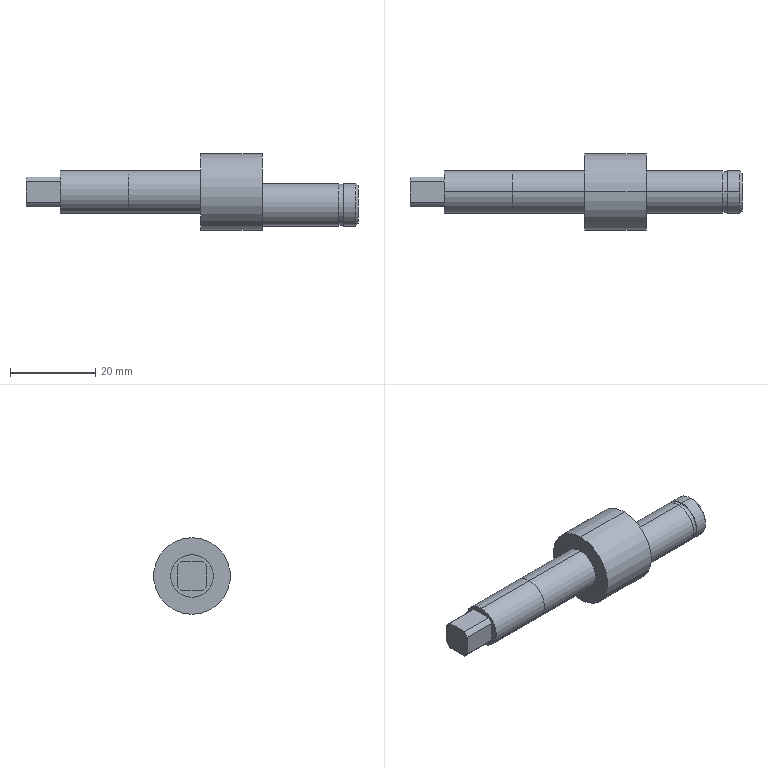Part | SolidWorks | features ICE 6, Chamfer 1, Extrusion 1 | 2 solids | 31 faces | box 78 x 18 x 18 mm | volume 8414 mm3 | cylinder 16 | plane 13 | cone 2 | commonest cylinder face diameters 10 x8 8.5 x4 9.6 x2 18 x2
STEP:
#1=CARTESIAN_POINT('',(-17.,0.,5.));
#2=VERTEX_POINT('',#1);
#3=CARTESIAN_POINT('',(-17.,0.,-5.));
#4=VERTEX_POINT('',#3);
#5=CARTESIAN_POINT('',(-17.,0.,0.));
#6=DIRECTION('',(-1.,0.,0.));
#7=DIRECTION('',(0.,0.,1.));
#8=AXIS2_PLACEMENT_3D('',#5,#6,#7);
#9=CIRCLE('',#8,5.);
#10=EDGE_CURVE('',#2,#4,#9,.T.);
#11=ORIENTED_EDGE('',*,*,#10,.F.);
#12=CARTESIAN_POINT('',(0.,0.,5.));
#13=VERTEX_POINT('',#12);
#14=CARTESIAN_POINT('',(-17.,0.,5.));
#15=DIRECTION('',(1.,0.,0.));
#16=VECTOR('',#15,1000.);
#17=LINE('',#14,#16);
#18=EDGE_CURVE('',#2,#13,#17,.T.);
#19=ORIENTED_EDGE('',*,*,#18,.T.);
#20=CARTESIAN_POINT('',(0.,0.,-5.));
#21=VERTEX_POINT('',#20);
#22=CARTESIAN_POINT('',(0.,0.,0.));
#23=DIRECTION('',(-1.,0.,0.));
#24=DIRECTION('',(0.,0.,1.));
#25=AXIS2_PLACEMENT_3D('',#22,#23,#24);
#26=CIRCLE('',#25,5.);
#27=EDGE_CURVE('',#13,#21,#26,.T.);
#28=ORIENTED_EDGE('',*,*,#27,.T.);
#29=CARTESIAN_POINT('',(-17.,0.,-5.));
#30=DIRECTION('',(1.,0.,0.));
#31=VECTOR('',#30,1000.);
#32=LINE('',#29,#31);
#33=EDGE_CURVE('',#4,#21,#32,.T.);
#34=ORIENTED_EDGE('',*,*,#33,.F.);
#35=EDGE_LOOP('',(#11,#19,#28,#34));
#36=FACE_OUTER_BOUND('',#35,.T.);
#37=CARTESIAN_POINT('',(-17.,0.,0.));
#38=DIRECTION('',(1.,0.,0.));
#39=DIRECTION('',(0.,0.,-1.));
#40=AXIS2_PLACEMENT_3D('',#37,#38,#39);
#41=CYLINDRICAL_SURFACE('',#40,5.);
#42=ADVANCED_FACE('',(#36),#41,.T.);
#43=CARTESIAN_POINT('',(37.,0.,-7.5));
#44=VERTEX_POINT('',#43);
#45=CARTESIAN_POINT('',(37.,0.,1.5));
#46=VERTEX_POINT('',#45);
#47=CARTESIAN_POINT('',(37.,0.,-3.));
#48=DIRECTION('',(1.,0.,0.));
#49=DIRECTION('',(0.,0.,-1.));
#50=AXIS2_PLACEMENT_3D('',#47,#48,#49);
#51=CIRCLE('',#50,4.5);
#52=EDGE_CURVE('',#44,#46,#51,.T.);
#53=ORIENTED_EDGE('',*,*,#52,.F.);
#54=CARTESIAN_POINT('',(36.5,0.,-8.));
#55=VERTEX_POINT('',#54);
#56=CARTESIAN_POINT('',(37.,0.,-7.5));
#57=DIRECTION('',(-0.7071,0.,-0.7071));
#58=VECTOR('',#57,1000.);
#59=LINE('',#56,#58);
#60=EDGE_CURVE('',#44,#55,#59,.T.);
#61=ORIENTED_EDGE('',*,*,#60,.T.);
#62=CARTESIAN_POINT('',(36.5,0.,2.));
#63=VERTEX_POINT('',#62);
#64=CARTESIAN_POINT('',(36.5,0.,-3.));
#65=DIRECTION('',(-1.,0.,0.));
#66=DIRECTION('',(0.,0.,-1.));
#67=AXIS2_PLACEMENT_3D('',#64,#65,#66);
#68=CIRCLE('',#67,5.);
#69=EDGE_CURVE('',#63,#55,#68,.T.);
#70=ORIENTED_EDGE('',*,*,#69,.F.);
#71=CARTESIAN_POINT('',(37.,0.,1.5));
#72=DIRECTION('',(-0.7071,0.,0.7071));
#73=VECTOR('',#72,1000.);
#74=LINE('',#71,#73);
#75=EDGE_CURVE('',#46,#63,#74,.T.);
#76=ORIENTED_EDGE('',*,*,#75,.F.);
#77=EDGE_LOOP('',(#53,#61,#70,#76));
#78=FACE_OUTER_BOUND('',#77,.T.);
#79=CARTESIAN_POINT('',(37.,0.,-3.));
#80=DIRECTION('',(-1.,0.,0.));
#81=DIRECTION('',(0.,0.,1.));
#82=AXIS2_PLACEMENT_3D('',#79,#80,#81);
#83=CONICAL_SURFACE('',#82,4.5,0.7854);
#84=ADVANCED_FACE('',(#78),#83,.T.);
#85=ORIENTED_EDGE('',*,*,#69,.T.);
#86=CARTESIAN_POINT('',(33.6,0.,-8.));
#87=VERTEX_POINT('',#86);
#88=CARTESIAN_POINT('',(37.,0.,-8.));
#89=DIRECTION('',(-1.,0.,0.));
#90=VECTOR('',#89,1000.);
#91=LINE('',#88,#90);
#92=EDGE_CURVE('',#55,#87,#91,.T.);
#93=ORIENTED_EDGE('',*,*,#92,.T.);
#94=CARTESIAN_POINT('',(33.6,0.,2.));
#95=VERTEX_POINT('',#94);
#96=CARTESIAN_POINT('',(33.6,0.,-3.));
#97=DIRECTION('',(1.,0.,0.));
#98=DIRECTION('',(0.,0.,-1.));
#99=AXIS2_PLACEMENT_3D('',#96,#97,#98);
#100=CIRCLE('',#99,5.);
#101=EDGE_CURVE('',#87,#95,#100,.T.);
#102=ORIENTED_EDGE('',*,*,#101,.T.);
#103=CARTESIAN_POINT('',(37.,0.,2.));
#104=DIRECTION('',(-1.,0.,0.));
#105=VECTOR('',#104,1000.);
#106=LINE('',#103,#105);
#107=EDGE_CURVE('',#63,#95,#106,.T.);
#108=ORIENTED_EDGE('',*,*,#107,.F.);
#109=EDGE_LOOP('',(#85,#93,#102,#108));
#110=FACE_OUTER_BOUND('',#109,.T.);
#111=CARTESIAN_POINT('',(37.,0.,-3.));
#112=DIRECTION('',(-1.,0.,0.));
#113=DIRECTION('',(0.,0.,1.));
#114=AXIS2_PLACEMENT_3D('',#111,#112,#113);
#115=CYLINDRICAL_SURFACE('',#114,5.);
#116=ADVANCED_FACE('',(#110),#115,.T.);
#117=CARTESIAN_POINT('',(33.6,0.,-7.8));
#118=VERTEX_POINT('',#117);
#119=CARTESIAN_POINT('',(33.6,0.,1.8));
#120=VERTEX_POINT('',#119);
#121=CARTESIAN_POINT('',(33.6,0.,-3.));
#122=DIRECTION('',(1.,0.,0.));
#123=DIRECTION('',(0.,0.,-1.));
#124=AXIS2_PLACEMENT_3D('',#121,#122,#123);
#125=CIRCLE('',#124,4.8);
#126=EDGE_CURVE('',#118,#120,#125,.T.);
#127=ORIENTED_EDGE('',*,*,#126,.F.);
#128=CARTESIAN_POINT('',(32.5,0.,-7.8));
#129=VERTEX_POINT('',#128);
#130=CARTESIAN_POINT('',(33.6,0.,-7.8));
#131=DIRECTION('',(-1.,0.,0.));
#132=VECTOR('',#131,1000.);
#133=LINE('',#130,#132);
#134=EDGE_CURVE('',#118,#129,#133,.T.);
#135=ORIENTED_EDGE('',*,*,#134,.T.);
#136=CARTESIAN_POINT('',(32.5,0.,1.8));
#137=VERTEX_POINT('',#136);
#138=CARTESIAN_POINT('',(32.5,0.,-3.));
#139=DIRECTION('',(1.,0.,0.));
#140=DIRECTION('',(0.,0.,-1.));
#141=AXIS2_PLACEMENT_3D('',#138,#139,#140);
#142=CIRCLE('',#141,4.8);
#143=EDGE_CURVE('',#129,#137,#142,.T.);
#144=ORIENTED_EDGE('',*,*,#143,.T.);
#145=CARTESIAN_POINT('',(33.6,0.,1.8));
#146=DIRECTION('',(-1.,0.,0.));
#147=VECTOR('',#146,1000.);
#148=LINE('',#145,#147);
#149=EDGE_CURVE('',#120,#137,#148,.T.);
#150=ORIENTED_EDGE('',*,*,#149,.F.);
#151=EDGE_LOOP('',(#127,#135,#144,#150));
#152=FACE_OUTER_BOUND('',#151,.T.);
#153=CARTESIAN_POINT('',(33.6,0.,-3.));
#154=DIRECTION('',(-1.,0.,0.));
#155=DIRECTION('',(0.,0.,1.));
#156=AXIS2_PLACEMENT_3D('',#153,#154,#155);
#157=CYLINDRICAL_SURFACE('',#156,4.8);
#158=ADVANCED_FACE('',(#152),#157,.T.);
#159=CARTESIAN_POINT('',(32.5,0.,-8.));
#160=VERTEX_POINT('',#159);
#161=CARTESIAN_POINT('',(32.5,0.,2.));
#162=VERTEX_POINT('',#161);
#163=CARTESIAN_POINT('',(32.5,0.,-3.));
#164=DIRECTION('',(1.,0.,0.));
#165=DIRECTION('',(0.,0.,-1.));
#166=AXIS2_PLACEMENT_3D('',#163,#164,#165);
#167=CIRCLE('',#166,5.);
#168=EDGE_CURVE('',#160,#162,#167,.T.);
#169=ORIENTED_EDGE('',*,*,#168,.F.);
#170=CARTESIAN_POINT('',(14.5,0.,-8.));
#171=VERTEX_POINT('',#170);
#172=CARTESIAN_POINT('',(32.5,0.,-8.));
#173=DIRECTION('',(-1.,0.,0.));
#174=VECTOR('',#173,1000.);
#175=LINE('',#172,#174);
#176=EDGE_CURVE('',#160,#171,#175,.T.);
#177=ORIENTED_EDGE('',*,*,#176,.T.);
#178=CARTESIAN_POINT('',(14.5,0.,2.));
#179=VERTEX_POINT('',#178);
#180=CARTESIAN_POINT('',(14.5,0.,-3.));
#181=DIRECTION('',(1.,0.,0.));
#182=DIRECTION('',(0.,0.,-1.));
#183=AXIS2_PLACEMENT_3D('',#180,#181,#182);
#184=CIRCLE('',#183,5.);
#185=EDGE_CURVE('',#171,#179,#184,.T.);
#186=ORIENTED_EDGE('',*,*,#185,.T.);
#187=CARTESIAN_POINT('',(32.5,0.,2.));
#188=DIRECTION('',(-1.,0.,0.));
#189=VECTOR('',#188,1000.);
#190=LINE('',#187,#189);
#191=EDGE_CURVE('',#162,#179,#190,.T.);
#192=ORIENTED_EDGE('',*,*,#191,.F.);
#193=EDGE_LOOP('',(#169,#177,#186,#192));
#194=FACE_OUTER_BOUND('',#193,.T.);
#195=CARTESIAN_POINT('',(32.5,0.,-3.));
#196=DIRECTION('',(-1.,0.,0.));
#197=DIRECTION('',(0.,0.,1.));
#198=AXIS2_PLACEMENT_3D('',#195,#196,#197);
#199=CYLINDRICAL_SURFACE('',#198,5.);
#200=ADVANCED_FACE('',(#194),#199,.T.);
#201=CARTESIAN_POINT('',(14.5,0.,-9.));
#202=VERTEX_POINT('',#201);
#203=CARTESIAN_POINT('',(14.5,0.,9.));
#204=VERTEX_POINT('',#203);
#205=CARTESIAN_POINT('',(14.5,0.,0.));
#206=DIRECTION('',(1.,0.,0.));
#207=DIRECTION('',(0.,0.,-1.));
#208=AXIS2_PLACEMENT_3D('',#205,#206,#207);
#209=CIRCLE('',#208,9.);
#210=EDGE_CURVE('',#202,#204,#209,.T.);
#211=ORIENTED_EDGE('',*,*,#210,.F.);
#212=CARTESIAN_POINT('',(0.,0.,-9.));
#213=VERTEX_POINT('',#212);
#214=CARTESIAN_POINT('',(14.5,0.,-9.));
#215=DIRECTION('',(-1.,0.,0.));
#216=VECTOR('',#215,1000.);
#217=LINE('',#214,#216);
#218=EDGE_CURVE('',#202,#213,#217,.T.);
#219=ORIENTED_EDGE('',*,*,#218,.T.);
#220=CARTESIAN_POINT('',(0.,0.,9.));
#221=VERTEX_POINT('',#220);
#222=CARTESIAN_POINT('',(0.,0.,0.));
#223=DIRECTION('',(1.,0.,0.));
#224=DIRECTION('',(0.,0.,-1.));
#225=AXIS2_PLACEMENT_3D('',#222,#223,#224);
#226=CIRCLE('',#225,9.);
#227=EDGE_CURVE('',#213,#221,#226,.T.);
#228=ORIENTED_EDGE('',*,*,#227,.T.);
#229=CARTESIAN_POINT('',(14.5,0.,9.));
#230=DIRECTION('',(-1.,0.,0.));
#231=VECTOR('',#230,1000.);
#232=LINE('',#229,#231);
#233=EDGE_CURVE('',#204,#221,#232,.T.);
#234=ORIENTED_EDGE('',*,*,#233,.F.);
#235=EDGE_LOOP('',(#211,#219,#228,#234));
#236=FACE_OUTER_BOUND('',#235,.T.);
#237=CARTESIAN_POINT('',(14.5,0.,0.));
#238=DIRECTION('',(-1.,0.,0.));
#239=DIRECTION('',(0.,0.,1.));
#240=AXIS2_PLACEMENT_3D('',#237,#238,#239);
#241=CYLINDRICAL_SURFACE('',#240,9.);
#242=ADVANCED_FACE('',(#236),#241,.T.);
#243=ORIENTED_EDGE('',*,*,#218,.F.);
#244=CARTESIAN_POINT('',(14.5,0.,0.));
#245=DIRECTION('',(1.,0.,0.));
#246=DIRECTION('',(0.,0.,-1.));
#247=AXIS2_PLACEMENT_3D('',#244,#245,#246);
#248=CIRCLE('',#247,9.);
#249=EDGE_CURVE('',#204,#202,#248,.T.);
#250=ORIENTED_EDGE('',*,*,#249,.F.);
#251=ORIENTED_EDGE('',*,*,#233,.T.);
#252=CARTESIAN_POINT('',(0.,0.,0.));
#253=DIRECTION('',(1.,0.,0.));
#254=DIRECTION('',(0.,0.,-1.));
#255=AXIS2_PLACEMENT_3D('',#252,#253,#254);
#256=CIRCLE('',#255,9.);
#257=EDGE_CURVE('',#221,#213,#256,.T.);
#258=ORIENTED_EDGE('',*,*,#257,.T.);
#259=EDGE_LOOP('',(#243,#250,#251,#258));
#260=FACE_OUTER_BOUND('',#259,.T.);
#261=CARTESIAN_POINT('',(14.5,0.,0.));
#262=DIRECTION('',(-1.,0.,0.));
#263=DIRECTION('',(0.,0.,1.));
#264=AXIS2_PLACEMENT_3D('',#261,#262,#263);
#265=CYLINDRICAL_SURFACE('',#264,9.);
#266=ADVANCED_FACE('',(#260),#265,.T.);
#267=CARTESIAN_POINT('',(14.5,0.,-3.));
#268=DIRECTION('',(1.,0.,0.));
#269=DIRECTION('',(0.,0.,-1.));
#270=AXIS2_PLACEMENT_3D('',#267,#268,#269);
#271=CIRCLE('',#270,5.);
#272=EDGE_CURVE('',#179,#171,#271,.T.);
#273=ORIENTED_EDGE('',*,*,#272,.F.);
#274=ORIENTED_EDGE('',*,*,#185,.F.);
#275=EDGE_LOOP('',(#273,#274));
#276=FACE_BOUND('',#275,.T.);
#277=ORIENTED_EDGE('',*,*,#249,.T.);
#278=ORIENTED_EDGE('',*,*,#210,.T.);
#279=EDGE_LOOP('',(#277,#278));
#280=FACE_OUTER_BOUND('',#279,.T.);
#281=CARTESIAN_POINT('',(14.5,0.,0.));
#282=DIRECTION('',(1.,0.,0.));
#283=DIRECTION('',(0.,0.,-1.));
#284=AXIS2_PLACEMENT_3D('',#281,#282,#283);
#285=PLANE('',#284);
#286=ADVANCED_FACE('',(#276,#280),#285,.T.);
#287=CARTESIAN_POINT('',(0.,0.,0.));
#288=DIRECTION('',(-1.,0.,0.));
#289=DIRECTION('',(0.,0.,1.));
#290=AXIS2_PLACEMENT_3D('',#287,#288,#289);
#291=CIRCLE('',#290,5.);
#292=EDGE_CURVE('',#21,#13,#291,.T.);
#293=ORIENTED_EDGE('',*,*,#292,.F.);
#294=ORIENTED_EDGE('',*,*,#27,.F.);
#295=EDGE_LOOP('',(#293,#294));
#296=FACE_BOUND('',#295,.T.);
#297=ORIENTED_EDGE('',*,*,#257,.F.);
#298=ORIENTED_EDGE('',*,*,#227,.F.);
#299=EDGE_LOOP('',(#297,#298));
#300=FACE_OUTER_BOUND('',#299,.T.);
#301=CARTESIAN_POINT('',(0.,0.,0.));
#302=DIRECTION('',(1.,0.,0.));
#303=DIRECTION('',(0.,0.,-1.));
#304=AXIS2_PLACEMENT_3D('',#301,#302,#303);
#305=PLANE('',#304);
#306=ADVANCED_FACE('',(#296,#300),#305,.F.);
#307=ORIENTED_EDGE('',*,*,#176,.F.);
#308=CARTESIAN_POINT('',(32.5,0.,-3.));
#309=DIRECTION('',(1.,0.,0.));
#310=DIRECTION('',(0.,0.,-1.));
#311=AXIS2_PLACEMENT_3D('',#308,#309,#310);
#312=CIRCLE('',#311,5.);
#313=EDGE_CURVE('',#162,#160,#312,.T.);
#314=ORIENTED_EDGE('',*,*,#313,.F.);
#315=ORIENTED_EDGE('',*,*,#191,.T.);
#316=ORIENTED_EDGE('',*,*,#272,.T.);
#317=EDGE_LOOP('',(#307,#314,#315,#316));
#318=FACE_OUTER_BOUND('',#317,.T.);
#319=CARTESIAN_POINT('',(32.5,0.,-3.));
#320=DIRECTION('',(-1.,0.,0.));
#321=DIRECTION('',(0.,0.,1.));
#322=AXIS2_PLACEMENT_3D('',#319,#320,#321);
#323=CYLINDRICAL_SURFACE('',#322,5.);
#324=ADVANCED_FACE('',(#318),#323,.T.);
#325=CARTESIAN_POINT('',(32.5,0.,-3.));
#326=DIRECTION('',(1.,0.,0.));
#327=DIRECTION('',(0.,0.,-1.));
#328=AXIS2_PLACEMENT_3D('',#325,#326,#327);
#329=CIRCLE('',#328,4.8);
#330=EDGE_CURVE('',#137,#129,#329,.T.);
#331=ORIENTED_EDGE('',*,*,#330,.F.);
#332=ORIENTED_EDGE('',*,*,#143,.F.);
#333=EDGE_LOOP('',(#331,#332));
#334=FACE_BOUND('',#333,.T.);
#335=ORIENTED_EDGE('',*,*,#313,.T.);
#336=ORIENTED_EDGE('',*,*,#168,.T.);
#337=EDGE_LOOP('',(#335,#336));
#338=FACE_OUTER_BOUND('',#337,.T.);
#339=CARTESIAN_POINT('',(32.5,0.,-3.));
#340=DIRECTION('',(1.,0.,0.));
#341=DIRECTION('',(0.,0.,-1.));
#342=AXIS2_PLACEMENT_3D('',#339,#340,#341);
#343=PLANE('',#342);
#344=ADVANCED_FACE('',(#334,#338),#343,.T.);
#345=ORIENTED_EDGE('',*,*,#134,.F.);
#346=CARTESIAN_POINT('',(33.6,0.,-3.));
#347=DIRECTION('',(1.,0.,0.));
#348=DIRECTION('',(0.,0.,-1.));
#349=AXIS2_PLACEMENT_3D('',#346,#347,#348);
#350=CIRCLE('',#349,4.8);
#351=EDGE_CURVE('',#120,#118,#350,.T.);
#352=ORIENTED_EDGE('',*,*,#351,.F.);
#353=ORIENTED_EDGE('',*,*,#149,.T.);
#354=ORIENTED_EDGE('',*,*,#330,.T.);
#355=EDGE_LOOP('',(#345,#352,#353,#354));
#356=FACE_OUTER_BOUND('',#355,.T.);
#357=CARTESIAN_POINT('',(33.6,0.,-3.));
#358=DIRECTION('',(-1.,0.,0.));
#359=DIRECTION('',(0.,0.,1.));
#360=AXIS2_PLACEMENT_3D('',#357,#358,#359);
#361=CYLINDRICAL_SURFACE('',#360,4.8);
#362=ADVANCED_FACE('',(#356),#361,.T.);
#363=ORIENTED_EDGE('',*,*,#92,.F.);
#364=CARTESIAN_POINT('',(36.5,0.,-3.));
#365=DIRECTION('',(-1.,0.,0.));
#366=DIRECTION('',(0.,0.,-1.));
#367=AXIS2_PLACEMENT_3D('',#364,#365,#366);
#368=CIRCLE('',#367,5.);
#369=EDGE_CURVE('',#55,#63,#368,.T.);
#370=ORIENTED_EDGE('',*,*,#369,.T.);
#371=ORIENTED_EDGE('',*,*,#107,.T.);
#372=CARTESIAN_POINT('',(33.6,0.,-3.));
#373=DIRECTION('',(1.,0.,0.));
#374=DIRECTION('',(0.,0.,-1.));
#375=AXIS2_PLACEMENT_3D('',#372,#373,#374);
#376=CIRCLE('',#375,5.);
#377=EDGE_CURVE('',#95,#87,#376,.T.);
#378=ORIENTED_EDGE('',*,*,#377,.T.);
#379=EDGE_LOOP('',(#363,#370,#371,#378));
#380=FACE_OUTER_BOUND('',#379,.T.);
#381=CARTESIAN_POINT('',(37.,0.,-3.));
#382=DIRECTION('',(-1.,0.,0.));
#383=DIRECTION('',(0.,0.,1.));
#384=AXIS2_PLACEMENT_3D('',#381,#382,#383);
#385=CYLINDRICAL_SURFACE('',#384,5.);
#386=ADVANCED_FACE('',(#380),#385,.T.);
#387=CARTESIAN_POINT('',(37.,0.,-3.));
#388=DIRECTION('',(1.,0.,0.));
#389=DIRECTION('',(0.,0.,-1.));
#390=AXIS2_PLACEMENT_3D('',#387,#388,#389);
#391=CIRCLE('',#390,4.5);
#392=EDGE_CURVE('',#46,#44,#391,.T.);
#393=ORIENTED_EDGE('',*,*,#392,.T.);
#394=ORIENTED_EDGE('',*,*,#52,.T.);
#395=EDGE_LOOP('',(#393,#394));
#396=FACE_OUTER_BOUND('',#395,.T.);
#397=CARTESIAN_POINT('',(37.,0.,-3.));
#398=DIRECTION('',(1.,0.,0.));
#399=DIRECTION('',(0.,0.,-1.));
#400=AXIS2_PLACEMENT_3D('',#397,#398,#399);
#401=PLANE('',#400);
#402=ADVANCED_FACE('',(#396),#401,.T.);
#403=ORIENTED_EDGE('',*,*,#351,.T.);
#404=ORIENTED_EDGE('',*,*,#126,.T.);
#405=EDGE_LOOP('',(#403,#404));
#406=FACE_BOUND('',#405,.T.);
#407=ORIENTED_EDGE('',*,*,#377,.F.);
#408=ORIENTED_EDGE('',*,*,#101,.F.);
#409=EDGE_LOOP('',(#407,#408));
#410=FACE_OUTER_BOUND('',#409,.T.);
#411=CARTESIAN_POINT('',(33.6,0.,-3.));
#412=DIRECTION('',(1.,0.,0.));
#413=DIRECTION('',(0.,0.,-1.));
#414=AXIS2_PLACEMENT_3D('',#411,#412,#413);
#415=PLANE('',#414);
#416=ADVANCED_FACE('',(#406,#410),#415,.F.);
#417=ORIENTED_EDGE('',*,*,#60,.F.);
#418=ORIENTED_EDGE('',*,*,#392,.F.);
#419=ORIENTED_EDGE('',*,*,#75,.T.);
#420=ORIENTED_EDGE('',*,*,#369,.F.);
#421=EDGE_LOOP('',(#417,#418,#419,#420));
#422=FACE_OUTER_BOUND('',#421,.T.);
#423=CARTESIAN_POINT('',(37.,0.,-3.));
#424=DIRECTION('',(-1.,0.,0.));
#425=DIRECTION('',(0.,0.,1.));
#426=AXIS2_PLACEMENT_3D('',#423,#424,#425);
#427=CONICAL_SURFACE('',#426,4.5,0.7854);
#428=ADVANCED_FACE('',(#422),#427,.T.);
#429=ORIENTED_EDGE('',*,*,#18,.F.);
#430=CARTESIAN_POINT('',(-17.,0.,0.));
#431=DIRECTION('',(-1.,0.,0.));
#432=DIRECTION('',(0.,0.,1.));
#433=AXIS2_PLACEMENT_3D('',#430,#431,#432);
#434=CIRCLE('',#433,5.);
#435=EDGE_CURVE('',#4,#2,#434,.T.);
#436=ORIENTED_EDGE('',*,*,#435,.F.);
#437=ORIENTED_EDGE('',*,*,#33,.T.);
#438=ORIENTED_EDGE('',*,*,#292,.T.);
#439=EDGE_LOOP('',(#429,#436,#437,#438));
#440=FACE_OUTER_BOUND('',#439,.T.);
#441=CARTESIAN_POINT('',(-17.,0.,0.));
#442=DIRECTION('',(1.,0.,0.));
#443=DIRECTION('',(0.,0.,-1.));
#444=AXIS2_PLACEMENT_3D('',#441,#442,#443);
#445=CYLINDRICAL_SURFACE('',#444,5.);
#446=ADVANCED_FACE('',(#440),#445,.T.);
#447=ORIENTED_EDGE('',*,*,#435,.T.);
#448=ORIENTED_EDGE('',*,*,#10,.T.);
#449=EDGE_LOOP('',(#447,#448));
#450=FACE_OUTER_BOUND('',#449,.T.);
#451=CARTESIAN_POINT('',(-17.,0.,0.));
#452=DIRECTION('',(-1.,0.,0.));
#453=DIRECTION('',(0.,0.,1.));
#454=AXIS2_PLACEMENT_3D('',#451,#452,#453);
#455=PLANE('',#454);
#456=ADVANCED_FACE('',(#450),#455,.T.);
#457=CLOSED_SHELL('',(#42,#84,#116,#158,#200,#242,#266,#286,#306,#324,#344,#362,#386,#402,#416,#428,#446,#456));
#458=MANIFOLD_SOLID_BREP('',#457);
#459=CARTESIAN_POINT('',(-33.,0.,5.));
#460=VERTEX_POINT('',#459);
#461=CARTESIAN_POINT('',(-33.,0.,-5.));
#462=VERTEX_POINT('',#461);
#463=CARTESIAN_POINT('',(-33.,0.,0.));
#464=DIRECTION('',(-1.,0.,0.));
#465=DIRECTION('',(0.,0.,1.));
#466=AXIS2_PLACEMENT_3D('',#463,#464,#465);
#467=CIRCLE('',#466,5.);
#468=EDGE_CURVE('',#460,#462,#467,.T.);
#469=ORIENTED_EDGE('',*,*,#468,.F.);
#470=CARTESIAN_POINT('',(-17.,0.,5.));
#471=VERTEX_POINT('',#470);
#472=CARTESIAN_POINT('',(-33.,0.,5.));
#473=DIRECTION('',(1.,0.,0.));
#474=VECTOR('',#473,1000.);
#475=LINE('',#472,#474);
#476=EDGE_CURVE('',#460,#471,#475,.T.);
#477=ORIENTED_EDGE('',*,*,#476,.T.);
#478=CARTESIAN_POINT('',(-17.,0.,-5.));
#479=VERTEX_POINT('',#478);
#480=CARTESIAN_POINT('',(-17.,0.,0.));
#481=DIRECTION('',(-1.,0.,0.));
#482=DIRECTION('',(0.,0.,1.));
#483=AXIS2_PLACEMENT_3D('',#480,#481,#482);
#484=CIRCLE('',#483,5.);
#485=EDGE_CURVE('',#471,#479,#484,.T.);
#486=ORIENTED_EDGE('',*,*,#485,.T.);
#487=CARTESIAN_POINT('',(-33.,0.,-5.));
#488=DIRECTION('',(1.,0.,0.));
#489=VECTOR('',#488,1000.);
#490=LINE('',#487,#489);
#491=EDGE_CURVE('',#462,#479,#490,.T.);
#492=ORIENTED_EDGE('',*,*,#491,.F.);
#493=EDGE_LOOP('',(#469,#477,#486,#492));
#494=FACE_OUTER_BOUND('',#493,.T.);
#495=CARTESIAN_POINT('',(-33.,0.,0.));
#496=DIRECTION('',(1.,0.,0.));
#497=DIRECTION('',(0.,0.,-1.));
#498=AXIS2_PLACEMENT_3D('',#495,#496,#497);
#499=CYLINDRICAL_SURFACE('',#498,5.);
#500=ADVANCED_FACE('',(#494),#499,.T.);
#501=ORIENTED_EDGE('',*,*,#476,.F.);
#502=CARTESIAN_POINT('',(-33.,0.,0.));
#503=DIRECTION('',(-1.,0.,0.));
#504=DIRECTION('',(0.,0.,1.));
#505=AXIS2_PLACEMENT_3D('',#502,#503,#504);
#506=CIRCLE('',#505,5.);
#507=EDGE_CURVE('',#462,#460,#506,.T.);
#508=ORIENTED_EDGE('',*,*,#507,.F.);
#509=ORIENTED_EDGE('',*,*,#491,.T.);
#510=CARTESIAN_POINT('',(-17.,0.,0.));
#511=DIRECTION('',(-1.,0.,0.));
#512=DIRECTION('',(0.,0.,1.));
#513=AXIS2_PLACEMENT_3D('',#510,#511,#512);
#514=CIRCLE('',#513,5.);
#515=EDGE_CURVE('',#479,#471,#514,.T.);
#516=ORIENTED_EDGE('',*,*,#515,.T.);
#517=EDGE_LOOP('',(#501,#508,#509,#516));
#518=FACE_OUTER_BOUND('',#517,.T.);
#519=CARTESIAN_POINT('',(-33.,0.,0.));
#520=DIRECTION('',(1.,0.,0.));
#521=DIRECTION('',(0.,0.,-1.));
#522=AXIS2_PLACEMENT_3D('',#519,#520,#521);
#523=CYLINDRICAL_SURFACE('',#522,5.);
#524=ADVANCED_FACE('',(#518),#523,.T.);
#525=CARTESIAN_POINT('',(-33.,3.5,-2.411));
#526=VERTEX_POINT('',#525);
#527=CARTESIAN_POINT('',(-33.,2.411,-3.5));
#528=VERTEX_POINT('',#527);
#529=CARTESIAN_POINT('',(-33.,0.,0.));
#530=DIRECTION('',(-1.,0.,0.));
#531=DIRECTION('',(0.,0.,1.));
#532=AXIS2_PLACEMENT_3D('',#529,#530,#531);
#533=CIRCLE('',#532,4.25);
#534=EDGE_CURVE('',#526,#528,#533,.T.);
#535=ORIENTED_EDGE('',*,*,#534,.F.);
#536=CARTESIAN_POINT('',(-33.,3.5,2.411));
#537=VERTEX_POINT('',#536);
#538=CARTESIAN_POINT('',(-33.,3.5,-2.411));
#539=DIRECTION('',(0.,0.,-1.));
#540=VECTOR('',#539,1000.);
#541=LINE('',#538,#540);
#542=EDGE_CURVE('',#537,#526,#541,.T.);
#543=ORIENTED_EDGE('',*,*,#542,.F.);
#544=CARTESIAN_POINT('',(-33.,2.411,3.5));
#545=VERTEX_POINT('',#544);
#546=CARTESIAN_POINT('',(-33.,0.,0.));
#547=DIRECTION('',(-1.,0.,0.));
#548=DIRECTION('',(0.,0.,1.));
#549=AXIS2_PLACEMENT_3D('',#546,#547,#548);
#550=CIRCLE('',#549,4.25);
#551=EDGE_CURVE('',#545,#537,#550,.T.);
#552=ORIENTED_EDGE('',*,*,#551,.F.);
#553=CARTESIAN_POINT('',(-33.,-2.411,3.5));
#554=VERTEX_POINT('',#553);
#555=CARTESIAN_POINT('',(-33.,-2.411,3.5));
#556=DIRECTION('',(0.,1.,0.));
#557=VECTOR('',#556,1000.);
#558=LINE('',#555,#557);
#559=EDGE_CURVE('',#554,#545,#558,.T.);
#560=ORIENTED_EDGE('',*,*,#559,.F.);
#561=CARTESIAN_POINT('',(-33.,-3.5,2.411));
#562=VERTEX_POINT('',#561);
#563=CARTESIAN_POINT('',(-33.,0.,0.));
#564=DIRECTION('',(-1.,0.,0.));
#565=DIRECTION('',(0.,0.,1.));
#566=AXIS2_PLACEMENT_3D('',#563,#564,#565);
#567=CIRCLE('',#566,4.25);
#568=EDGE_CURVE('',#562,#554,#567,.T.);
#569=ORIENTED_EDGE('',*,*,#568,.F.);
#570=CARTESIAN_POINT('',(-33.,-3.5,-2.411));
#571=VERTEX_POINT('',#570);
#572=CARTESIAN_POINT('',(-33.,-3.5,-2.411));
#573=DIRECTION('',(0.,0.,1.));
#574=VECTOR('',#573,1000.);
#575=LINE('',#572,#574);
#576=EDGE_CURVE('',#571,#562,#575,.T.);
#577=ORIENTED_EDGE('',*,*,#576,.F.);
#578=CARTESIAN_POINT('',(-33.,-2.411,-3.5));
#579=VERTEX_POINT('',#578);
#580=CARTESIAN_POINT('',(-33.,0.,0.));
#581=DIRECTION('',(-1.,0.,0.));
#582=DIRECTION('',(0.,0.,1.));
#583=AXIS2_PLACEMENT_3D('',#580,#581,#582);
#584=CIRCLE('',#583,4.25);
#585=EDGE_CURVE('',#579,#571,#584,.T.);
#586=ORIENTED_EDGE('',*,*,#585,.F.);
#587=CARTESIAN_POINT('',(-33.,-2.411,-3.5));
#588=DIRECTION('',(0.,-1.,0.));
#589=VECTOR('',#588,1000.);
#590=LINE('',#587,#589);
#591=EDGE_CURVE('',#528,#579,#590,.T.);
#592=ORIENTED_EDGE('',*,*,#591,.F.);
#593=EDGE_LOOP('',(#535,#543,#552,#560,#569,#577,#586,#592));
#594=FACE_BOUND('',#593,.T.);
#595=ORIENTED_EDGE('',*,*,#507,.T.);
#596=ORIENTED_EDGE('',*,*,#468,.T.);
#597=EDGE_LOOP('',(#595,#596));
#598=FACE_OUTER_BOUND('',#597,.T.);
#599=CARTESIAN_POINT('',(-33.,0.,0.));
#600=DIRECTION('',(-1.,0.,0.));
#601=DIRECTION('',(0.,0.,1.));
#602=AXIS2_PLACEMENT_3D('',#599,#600,#601);
#603=PLANE('',#602);
#604=ADVANCED_FACE('',(#594,#598),#603,.T.);
#605=ORIENTED_EDGE('',*,*,#515,.F.);
#606=ORIENTED_EDGE('',*,*,#485,.F.);
#607=EDGE_LOOP('',(#605,#606));
#608=FACE_OUTER_BOUND('',#607,.T.);
#609=CARTESIAN_POINT('',(-17.,0.,0.));
#610=DIRECTION('',(-1.,0.,0.));
#611=DIRECTION('',(0.,0.,1.));
#612=AXIS2_PLACEMENT_3D('',#609,#610,#611);
#613=PLANE('',#612);
#614=ADVANCED_FACE('',(#608),#613,.F.);
#615=ORIENTED_EDGE('',*,*,#534,.T.);
#616=CARTESIAN_POINT('',(-41.,2.411,-3.5));
#617=VERTEX_POINT('',#616);
#618=CARTESIAN_POINT('',(-41.,2.411,-3.5));
#619=DIRECTION('',(1.,0.,0.));
#620=VECTOR('',#619,1000.);
#621=LINE('',#618,#620);
#622=EDGE_CURVE('',#617,#528,#621,.T.);
#623=ORIENTED_EDGE('',*,*,#622,.F.);
#624=CARTESIAN_POINT('',(-41.,3.5,-2.411));
#625=VERTEX_POINT('',#624);
#626=CARTESIAN_POINT('',(-41.,0.,0.));
#627=DIRECTION('',(-1.,0.,0.));
#628=DIRECTION('',(0.,0.,1.));
#629=AXIS2_PLACEMENT_3D('',#626,#627,#628);
#630=CIRCLE('',#629,4.25);
#631=EDGE_CURVE('',#625,#617,#630,.T.);
#632=ORIENTED_EDGE('',*,*,#631,.F.);
#633=CARTESIAN_POINT('',(-41.,3.5,-2.411));
#634=DIRECTION('',(1.,0.,0.));
#635=VECTOR('',#634,1000.);
#636=LINE('',#633,#635);
#637=EDGE_CURVE('',#625,#526,#636,.T.);
#638=ORIENTED_EDGE('',*,*,#637,.T.);
#639=EDGE_LOOP('',(#615,#623,#632,#638));
#640=FACE_OUTER_BOUND('',#639,.T.);
#641=CARTESIAN_POINT('',(-41.,0.,0.));
#642=DIRECTION('',(1.,0.,0.));
#643=DIRECTION('',(0.,0.,-1.));
#644=AXIS2_PLACEMENT_3D('',#641,#642,#643);
#645=CYLINDRICAL_SURFACE('',#644,4.25);
#646=ADVANCED_FACE('',(#640),#645,.T.);
#647=ORIENTED_EDGE('',*,*,#591,.T.);
#648=CARTESIAN_POINT('',(-41.,-2.411,-3.5));
#649=VERTEX_POINT('',#648);
#650=CARTESIAN_POINT('',(-41.,-2.411,-3.5));
#651=DIRECTION('',(1.,0.,0.));
#652=VECTOR('',#651,1000.);
#653=LINE('',#650,#652);
#654=EDGE_CURVE('',#649,#579,#653,.T.);
#655=ORIENTED_EDGE('',*,*,#654,.F.);
#656=CARTESIAN_POINT('',(-41.,-2.411,-3.5));
#657=DIRECTION('',(0.,-1.,0.));
#658=VECTOR('',#657,1000.);
#659=LINE('',#656,#658);
#660=EDGE_CURVE('',#617,#649,#659,.T.);
#661=ORIENTED_EDGE('',*,*,#660,.F.);
#662=ORIENTED_EDGE('',*,*,#622,.T.);
#663=EDGE_LOOP('',(#647,#655,#661,#662));
#664=FACE_OUTER_BOUND('',#663,.T.);
#665=CARTESIAN_POINT('',(-41.,-2.411,-3.5));
#666=DIRECTION('',(0.,0.,1.));
#667=DIRECTION('',(1.,0.,0.));
#668=AXIS2_PLACEMENT_3D('',#665,#666,#667);
#669=PLANE('',#668);
#670=ADVANCED_FACE('',(#664),#669,.F.);
#671=ORIENTED_EDGE('',*,*,#585,.T.);
#672=CARTESIAN_POINT('',(-41.,-3.5,-2.411));
#673=VERTEX_POINT('',#672);
#674=CARTESIAN_POINT('',(-41.,-3.5,-2.411));
#675=DIRECTION('',(1.,0.,0.));
#676=VECTOR('',#675,1000.);
#677=LINE('',#674,#676);
#678=EDGE_CURVE('',#673,#571,#677,.T.);
#679=ORIENTED_EDGE('',*,*,#678,.F.);
#680=CARTESIAN_POINT('',(-41.,0.,0.));
#681=DIRECTION('',(-1.,0.,0.));
#682=DIRECTION('',(0.,0.,1.));
#683=AXIS2_PLACEMENT_3D('',#680,#681,#682);
#684=CIRCLE('',#683,4.25);
#685=EDGE_CURVE('',#649,#673,#684,.T.);
#686=ORIENTED_EDGE('',*,*,#685,.F.);
#687=ORIENTED_EDGE('',*,*,#654,.T.);
#688=EDGE_LOOP('',(#671,#679,#686,#687));
#689=FACE_OUTER_BOUND('',#688,.T.);
#690=CARTESIAN_POINT('',(-41.,0.,0.));
#691=DIRECTION('',(1.,0.,0.));
#692=DIRECTION('',(0.,0.,-1.));
#693=AXIS2_PLACEMENT_3D('',#690,#691,#692);
#694=CYLINDRICAL_SURFACE('',#693,4.25);
#695=ADVANCED_FACE('',(#689),#694,.T.);
#696=ORIENTED_EDGE('',*,*,#576,.T.);
#697=CARTESIAN_POINT('',(-41.,-3.5,2.411));
#698=VERTEX_POINT('',#697);
#699=CARTESIAN_POINT('',(-41.,-3.5,2.411));
#700=DIRECTION('',(1.,0.,0.));
#701=VECTOR('',#700,1000.);
#702=LINE('',#699,#701);
#703=EDGE_CURVE('',#698,#562,#702,.T.);
#704=ORIENTED_EDGE('',*,*,#703,.F.);
#705=CARTESIAN_POINT('',(-41.,-3.5,-2.411));
#706=DIRECTION('',(0.,0.,1.));
#707=VECTOR('',#706,1000.);
#708=LINE('',#705,#707);
#709=EDGE_CURVE('',#673,#698,#708,.T.);
#710=ORIENTED_EDGE('',*,*,#709,.F.);
#711=ORIENTED_EDGE('',*,*,#678,.T.);
#712=EDGE_LOOP('',(#696,#704,#710,#711));
#713=FACE_OUTER_BOUND('',#712,.T.);
#714=CARTESIAN_POINT('',(-41.,-3.5,-2.411));
#715=DIRECTION('',(0.,1.,0.));
#716=DIRECTION('',(0.,0.,1.));
#717=AXIS2_PLACEMENT_3D('',#714,#715,#716);
#718=PLANE('',#717);
#719=ADVANCED_FACE('',(#713),#718,.F.);
#720=ORIENTED_EDGE('',*,*,#568,.T.);
#721=CARTESIAN_POINT('',(-41.,-2.411,3.5));
#722=VERTEX_POINT('',#721);
#723=CARTESIAN_POINT('',(-41.,-2.411,3.5));
#724=DIRECTION('',(1.,0.,0.));
#725=VECTOR('',#724,1000.);
#726=LINE('',#723,#725);
#727=EDGE_CURVE('',#722,#554,#726,.T.);
#728=ORIENTED_EDGE('',*,*,#727,.F.);
#729=CARTESIAN_POINT('',(-41.,0.,0.));
#730=DIRECTION('',(-1.,0.,0.));
#731=DIRECTION('',(0.,0.,1.));
#732=AXIS2_PLACEMENT_3D('',#729,#730,#731);
#733=CIRCLE('',#732,4.25);
#734=EDGE_CURVE('',#698,#722,#733,.T.);
#735=ORIENTED_EDGE('',*,*,#734,.F.);
#736=ORIENTED_EDGE('',*,*,#703,.T.);
#737=EDGE_LOOP('',(#720,#728,#735,#736));
#738=FACE_OUTER_BOUND('',#737,.T.);
#739=CARTESIAN_POINT('',(-41.,0.,0.));
#740=DIRECTION('',(1.,0.,0.));
#741=DIRECTION('',(0.,0.,-1.));
#742=AXIS2_PLACEMENT_3D('',#739,#740,#741);
#743=CYLINDRICAL_SURFACE('',#742,4.25);
#744=ADVANCED_FACE('',(#738),#743,.T.);
#745=ORIENTED_EDGE('',*,*,#559,.T.);
#746=CARTESIAN_POINT('',(-41.,2.411,3.5));
#747=VERTEX_POINT('',#746);
#748=CARTESIAN_POINT('',(-41.,2.411,3.5));
#749=DIRECTION('',(1.,0.,0.));
#750=VECTOR('',#749,1000.);
#751=LINE('',#748,#750);
#752=EDGE_CURVE('',#747,#545,#751,.T.);
#753=ORIENTED_EDGE('',*,*,#752,.F.);
#754=CARTESIAN_POINT('',(-41.,-2.411,3.5));
#755=DIRECTION('',(0.,1.,0.));
#756=VECTOR('',#755,1000.);
#757=LINE('',#754,#756);
#758=EDGE_CURVE('',#722,#747,#757,.T.);
#759=ORIENTED_EDGE('',*,*,#758,.F.);
#760=ORIENTED_EDGE('',*,*,#727,.T.);
#761=EDGE_LOOP('',(#745,#753,#759,#760));
#762=FACE_OUTER_BOUND('',#761,.T.);
#763=CARTESIAN_POINT('',(-41.,-2.411,3.5));
#764=DIRECTION('',(0.,0.,-1.));
#765=DIRECTION('',(-1.,0.,0.));
#766=AXIS2_PLACEMENT_3D('',#763,#764,#765);
#767=PLANE('',#766);
#768=ADVANCED_FACE('',(#762),#767,.F.);
#769=ORIENTED_EDGE('',*,*,#551,.T.);
#770=CARTESIAN_POINT('',(-41.,3.5,2.411));
#771=VERTEX_POINT('',#770);
#772=CARTESIAN_POINT('',(-41.,3.5,2.411));
#773=DIRECTION('',(1.,0.,0.));
#774=VECTOR('',#773,1000.);
#775=LINE('',#772,#774);
#776=EDGE_CURVE('',#771,#537,#775,.T.);
#777=ORIENTED_EDGE('',*,*,#776,.F.);
#778=CARTESIAN_POINT('',(-41.,0.,0.));
#779=DIRECTION('',(-1.,0.,0.));
#780=DIRECTION('',(0.,0.,1.));
#781=AXIS2_PLACEMENT_3D('',#778,#779,#780);
#782=CIRCLE('',#781,4.25);
#783=EDGE_CURVE('',#747,#771,#782,.T.);
#784=ORIENTED_EDGE('',*,*,#783,.F.);
#785=ORIENTED_EDGE('',*,*,#752,.T.);
#786=EDGE_LOOP('',(#769,#777,#784,#785));
#787=FACE_OUTER_BOUND('',#786,.T.);
#788=CARTESIAN_POINT('',(-41.,0.,0.));
#789=DIRECTION('',(1.,0.,0.));
#790=DIRECTION('',(0.,0.,-1.));
#791=AXIS2_PLACEMENT_3D('',#788,#789,#790);
#792=CYLINDRICAL_SURFACE('',#791,4.25);
#793=ADVANCED_FACE('',(#787),#792,.T.);
#794=ORIENTED_EDGE('',*,*,#542,.T.);
#795=ORIENTED_EDGE('',*,*,#637,.F.);
#796=CARTESIAN_POINT('',(-41.,3.5,-2.411));
#797=DIRECTION('',(0.,0.,-1.));
#798=VECTOR('',#797,1000.);
#799=LINE('',#796,#798);
#800=EDGE_CURVE('',#771,#625,#799,.T.);
#801=ORIENTED_EDGE('',*,*,#800,.F.);
#802=ORIENTED_EDGE('',*,*,#776,.T.);
#803=EDGE_LOOP('',(#794,#795,#801,#802));
#804=FACE_OUTER_BOUND('',#803,.T.);
#805=CARTESIAN_POINT('',(-41.,3.5,-2.411));
#806=DIRECTION('',(0.,-1.,0.));
#807=DIRECTION('',(0.,0.,-1.));
#808=AXIS2_PLACEMENT_3D('',#805,#806,#807);
#809=PLANE('',#808);
#810=ADVANCED_FACE('',(#804),#809,.F.);
#811=ORIENTED_EDGE('',*,*,#631,.T.);
#812=ORIENTED_EDGE('',*,*,#660,.T.);
#813=ORIENTED_EDGE('',*,*,#685,.T.);
#814=ORIENTED_EDGE('',*,*,#709,.T.);
#815=ORIENTED_EDGE('',*,*,#734,.T.);
#816=ORIENTED_EDGE('',*,*,#758,.T.);
#817=ORIENTED_EDGE('',*,*,#783,.T.);
#818=ORIENTED_EDGE('',*,*,#800,.T.);
#819=EDGE_LOOP('',(#811,#812,#813,#814,#815,#816,#817,#818));
#820=FACE_OUTER_BOUND('',#819,.T.);
#821=CARTESIAN_POINT('',(-41.,0.,0.));
#822=DIRECTION('',(-1.,0.,0.));
#823=DIRECTION('',(0.,0.,1.));
#824=AXIS2_PLACEMENT_3D('',#821,#822,#823);
#825=PLANE('',#824);
#826=ADVANCED_FACE('',(#820),#825,.T.);
#827=CLOSED_SHELL('',(#500,#524,#604,#614,#646,#670,#695,#719,#744,#768,#793,#810,#826));
#828=MANIFOLD_SOLID_BREP('',#827);
#829=CARTESIAN_POINT('',(0.,0.,0.));
#830=DIRECTION('',(0.,0.,1.));
#831=DIRECTION('',(1.,0.,0.));
#832=AXIS2_PLACEMENT_3D('',#829,#830,#831);
#833=(LENGTH_UNIT()NAMED_UNIT(*)SI_UNIT(.MILLI.,.METRE.));
#834=UNCERTAINTY_MEASURE_WITH_UNIT(LENGTH_MEASURE(0.00001),#833,'','');
#835=(NAMED_UNIT(*)PLANE_ANGLE_UNIT()SI_UNIT($,.RADIAN.));
#836=(NAMED_UNIT(*)SI_UNIT($,.STERADIAN.)SOLID_ANGLE_UNIT());
#837=(GEOMETRIC_REPRESENTATION_CONTEXT(3)GLOBAL_UNCERTAINTY_ASSIGNED_CONTEXT((#834))GLOBAL_UNIT_ASSIGNED_CONTEXT((#833,#835,#836))REPRESENTATION_CONTEXT('',''));
#838=ADVANCED_BREP_SHAPE_REPRESENTATION('',(#458,#828,#832),#837);